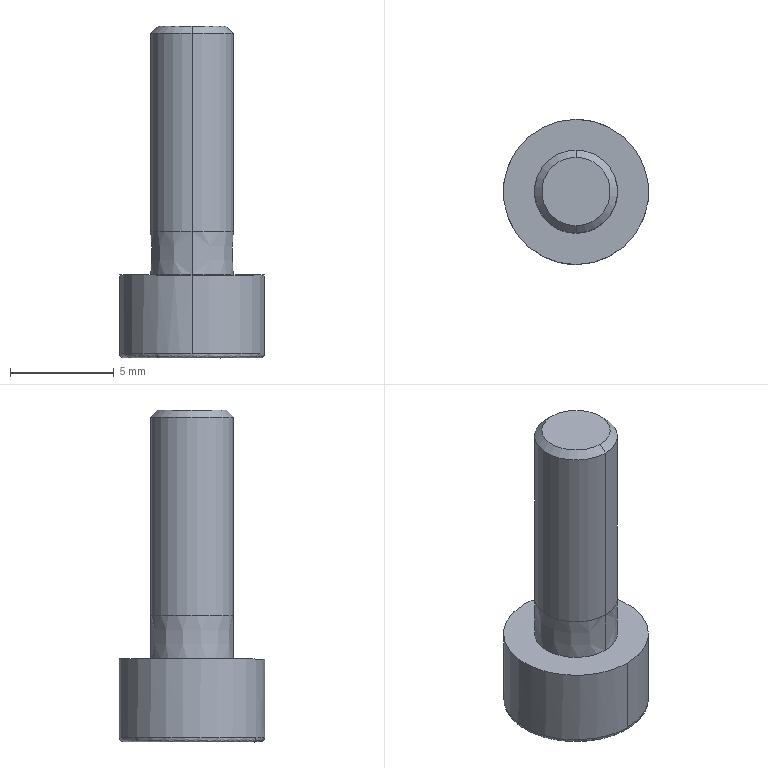Part | SolidWorks | features BaseBody 1 | 1 solid | 20 faces | box 7 x 7 x 16 mm | volume 288.226 mm3 | plane 10 | cylinder 4 | cone 4 | spline 2 | commonest cylinder face diameters 4 x2 7 x2
STEP:
#1=CARTESIAN_POINT('',(490.946,-51.279,245.744));
#2=VERTEX_POINT('',#1);
#3=CARTESIAN_POINT('',(489.266,-50.849,245.744));
#4=VERTEX_POINT('',#3);
#5=CARTESIAN_POINT('',(489.266,-54.349,245.744));
#6=DIRECTION('',(0.000000004,-0.00000001,1.));
#7=DIRECTION('',(0.,-1.,-0.00000001));
#8=AXIS2_PLACEMENT_3D('',#5,#6,#7);
#9=CIRCLE('',#8,3.5);
#10=EDGE_CURVE('',#2,#4,#9,.T.);
#11=ORIENTED_EDGE('',*,*,#10,.F.);
#12=CARTESIAN_POINT('',(490.85,-51.454,245.544));
#13=VERTEX_POINT('',#12);
#14=CARTESIAN_POINT('',(490.85,-51.454,245.744));
#15=DIRECTION('',(-0.8773,0.4799,0.000000008));
#16=DIRECTION('',(0.4799,0.8773,0.000000006));
#17=AXIS2_PLACEMENT_3D('',#14,#15,#16);
#18=CIRCLE('',#17,0.2);
#19=EDGE_CURVE('',#2,#13,#18,.T.);
#20=ORIENTED_EDGE('',*,*,#19,.T.);
#21=CARTESIAN_POINT('',(487.682,-57.244,245.544));
#22=VERTEX_POINT('',#21);
#23=CARTESIAN_POINT('',(490.85,-51.454,245.544));
#24=CARTESIAN_POINT('',(485.059,-48.287,245.544));
#25=CARTESIAN_POINT('',(481.892,-54.077,245.544));
#26=CARTESIAN_POINT('',(487.682,-57.244,245.544));
#27=(BOUNDED_CURVE()B_SPLINE_CURVE(3,(#23,#24,#25,#26),.UNSPECIFIED.,.F.,.T.)B_SPLINE_CURVE_WITH_KNOTS((4,4),(0.,1.),.UNSPECIFIED.)CURVE()GEOMETRIC_REPRESENTATION_ITEM()RATIONAL_B_SPLINE_CURVE((1.,0.3333,0.3333,1.))REPRESENTATION_ITEM(''));
#28=EDGE_CURVE('',#13,#22,#27,.T.);
#29=ORIENTED_EDGE('',*,*,#28,.T.);
#30=CARTESIAN_POINT('',(487.586,-57.42,245.744));
#31=VERTEX_POINT('',#30);
#32=CARTESIAN_POINT('',(487.682,-57.244,245.744));
#33=DIRECTION('',(0.8773,-0.4799,-0.000000008));
#34=DIRECTION('',(-0.4799,-0.8773,-0.000000006));
#35=AXIS2_PLACEMENT_3D('',#32,#33,#34);
#36=CIRCLE('',#35,0.2);
#37=EDGE_CURVE('',#31,#22,#36,.T.);
#38=ORIENTED_EDGE('',*,*,#37,.F.);
#39=CARTESIAN_POINT('',(489.266,-54.349,245.744));
#40=DIRECTION('',(0.000000004,-0.00000001,1.));
#41=DIRECTION('',(0.,-1.,-0.00000001));
#42=AXIS2_PLACEMENT_3D('',#39,#40,#41);
#43=CIRCLE('',#42,3.5);
#44=EDGE_CURVE('',#4,#31,#43,.T.);
#45=ORIENTED_EDGE('',*,*,#44,.F.);
#46=EDGE_LOOP('',(#11,#20,#29,#38,#45));
#47=FACE_OUTER_BOUND('',#46,.T.);
#48=CARTESIAN_POINT('',(490.946,-51.279,245.744));
#49=CARTESIAN_POINT('',(484.804,-47.919,245.744));
#50=CARTESIAN_POINT('',(481.445,-54.06,245.744));
#51=CARTESIAN_POINT('',(487.586,-57.42,245.744));
#52=CARTESIAN_POINT('',(490.946,-51.279,245.627));
#53=CARTESIAN_POINT('',(484.804,-47.919,245.627));
#54=CARTESIAN_POINT('',(481.445,-54.06,245.627));
#55=CARTESIAN_POINT('',(487.586,-57.42,245.627));
#56=CARTESIAN_POINT('',(490.906,-51.351,245.544));
#57=CARTESIAN_POINT('',(484.91,-48.071,245.544));
#58=CARTESIAN_POINT('',(481.63,-54.067,245.544));
#59=CARTESIAN_POINT('',(487.626,-57.347,245.544));
#60=CARTESIAN_POINT('',(490.85,-51.454,245.544));
#61=CARTESIAN_POINT('',(485.059,-48.287,245.544));
#62=CARTESIAN_POINT('',(481.892,-54.077,245.544));
#63=CARTESIAN_POINT('',(487.682,-57.244,245.544));
#64=(BOUNDED_SURFACE()B_SPLINE_SURFACE(3,3,((#48,#49,#50,#51),(#52,#53,#54,#55),(#56,#57,#58,#59),(#60,#61,#62,#63)),.UNSPECIFIED.,.F.,.F.,.F.)B_SPLINE_SURFACE_WITH_KNOTS((4,4),(4,4),(0.,1.),(0.,1.),.UNSPECIFIED.)GEOMETRIC_REPRESENTATION_ITEM()RATIONAL_B_SPLINE_SURFACE(((1.,0.3333,0.3333,1.),(0.8047,0.2682,0.2682,0.8047),(0.8047,0.2682,0.2682,0.8047),(1.,0.3333,0.3333,1.)))REPRESENTATION_ITEM('')SURFACE());
#65=ADVANCED_FACE('',(#47),#64,.T.);
#66=CARTESIAN_POINT('',(489.266,-56.349,251.644));
#67=VERTEX_POINT('',#66);
#68=CARTESIAN_POINT('',(489.266,-52.349,251.644));
#69=VERTEX_POINT('',#68);
#70=CARTESIAN_POINT('',(489.266,-54.349,251.644));
#71=DIRECTION('',(0.000000004,-0.00000001,1.));
#72=DIRECTION('',(0.,-1.,-0.00000001));
#73=AXIS2_PLACEMENT_3D('',#70,#71,#72);
#74=CIRCLE('',#73,2.);
#75=EDGE_CURVE('',#67,#69,#74,.T.);
#76=ORIENTED_EDGE('',*,*,#75,.T.);
#77=CARTESIAN_POINT('',(489.266,-52.349,261.194));
#78=VERTEX_POINT('',#77);
#79=CARTESIAN_POINT('',(489.266,-52.349,256.419));
#80=DIRECTION('',(0.000000004,-0.00000001,1.));
#81=VECTOR('',#80,1000.);
#82=LINE('',#79,#81);
#83=EDGE_CURVE('',#69,#78,#82,.T.);
#84=ORIENTED_EDGE('',*,*,#83,.T.);
#85=CARTESIAN_POINT('',(489.266,-56.349,261.194));
#86=VERTEX_POINT('',#85);
#87=CARTESIAN_POINT('',(489.266,-54.349,261.194));
#88=DIRECTION('',(-0.000000004,0.00000001,-1.));
#89=DIRECTION('',(0.,-1.,-0.00000001));
#90=AXIS2_PLACEMENT_3D('',#87,#88,#89);
#91=CIRCLE('',#90,2.);
#92=EDGE_CURVE('',#78,#86,#91,.T.);
#93=ORIENTED_EDGE('',*,*,#92,.T.);
#94=CARTESIAN_POINT('',(489.266,-56.349,256.419));
#95=DIRECTION('',(0.000000004,-0.00000001,1.));
#96=VECTOR('',#95,1000.);
#97=LINE('',#94,#96);
#98=EDGE_CURVE('',#67,#86,#97,.T.);
#99=ORIENTED_EDGE('',*,*,#98,.F.);
#100=EDGE_LOOP('',(#76,#84,#93,#99));
#101=FACE_OUTER_BOUND('',#100,.T.);
#102=CARTESIAN_POINT('',(489.266,-54.349,256.419));
#103=DIRECTION('',(0.000000004,-0.00000001,1.));
#104=DIRECTION('',(0.,-1.,-0.00000001));
#105=AXIS2_PLACEMENT_3D('',#102,#103,#104);
#106=CYLINDRICAL_SURFACE('',#105,2.);
#107=ADVANCED_FACE('',(#101),#106,.T.);
#108=CARTESIAN_POINT('',(489.266,-56.348,249.544));
#109=VERTEX_POINT('',#108);
#110=CARTESIAN_POINT('',(489.266,-52.35,249.544));
#111=VERTEX_POINT('',#110);
#112=CARTESIAN_POINT('',(489.266,-54.349,249.544));
#113=DIRECTION('',(0.000000004,-0.00000001,1.));
#114=DIRECTION('',(0.,-1.,-0.00000001));
#115=AXIS2_PLACEMENT_3D('',#112,#113,#114);
#116=CIRCLE('',#115,1.999);
#117=EDGE_CURVE('',#109,#111,#116,.T.);
#118=ORIENTED_EDGE('',*,*,#117,.T.);
#119=CARTESIAN_POINT('',(489.266,-52.349,251.644));
#120=DIRECTION('',(0.000000004,0.0004762,1.));
#121=VECTOR('',#120,1000.);
#122=LINE('',#119,#121);
#123=EDGE_CURVE('',#111,#69,#122,.T.);
#124=ORIENTED_EDGE('',*,*,#123,.T.);
#125=ORIENTED_EDGE('',*,*,#75,.F.);
#126=CARTESIAN_POINT('',(489.266,-56.349,251.644));
#127=DIRECTION('',(0.000000004,-0.0004762,1.));
#128=VECTOR('',#127,1000.);
#129=LINE('',#126,#128);
#130=EDGE_CURVE('',#109,#67,#129,.T.);
#131=ORIENTED_EDGE('',*,*,#130,.F.);
#132=EDGE_LOOP('',(#118,#124,#125,#131));
#133=FACE_OUTER_BOUND('',#132,.T.);
#134=CARTESIAN_POINT('',(489.266,-54.349,251.644));
#135=DIRECTION('',(0.000000004,-0.00000001,1.));
#136=DIRECTION('',(0.,-1.,-0.00000001));
#137=AXIS2_PLACEMENT_3D('',#134,#135,#136);
#138=CONICAL_SURFACE('',#137,2.,0.0004762);
#139=ADVANCED_FACE('',(#133),#138,.T.);
#140=CARTESIAN_POINT('',(489.266,-52.699,261.544));
#141=VERTEX_POINT('',#140);
#142=CARTESIAN_POINT('',(489.266,-55.999,261.544));
#143=VERTEX_POINT('',#142);
#144=CARTESIAN_POINT('',(489.266,-54.349,261.544));
#145=DIRECTION('',(-0.000000004,0.00000001,-1.));
#146=DIRECTION('',(0.,1.,0.00000001));
#147=AXIS2_PLACEMENT_3D('',#144,#145,#146);
#148=CIRCLE('',#147,1.65);
#149=EDGE_CURVE('',#141,#143,#148,.T.);
#150=ORIENTED_EDGE('',*,*,#149,.T.);
#151=CARTESIAN_POINT('',(489.266,-56.349,261.194));
#152=DIRECTION('',(-0.000000003,-0.7071,-0.7071));
#153=VECTOR('',#152,1000.);
#154=LINE('',#151,#153);
#155=EDGE_CURVE('',#143,#86,#154,.T.);
#156=ORIENTED_EDGE('',*,*,#155,.T.);
#157=ORIENTED_EDGE('',*,*,#92,.F.);
#158=CARTESIAN_POINT('',(489.266,-52.349,261.194));
#159=DIRECTION('',(-0.000000003,0.7071,-0.7071));
#160=VECTOR('',#159,1000.);
#161=LINE('',#158,#160);
#162=EDGE_CURVE('',#141,#78,#161,.T.);
#163=ORIENTED_EDGE('',*,*,#162,.F.);
#164=EDGE_LOOP('',(#150,#156,#157,#163));
#165=FACE_OUTER_BOUND('',#164,.T.);
#166=CARTESIAN_POINT('',(489.266,-54.349,261.194));
#167=DIRECTION('',(-0.000000004,0.00000001,-1.));
#168=DIRECTION('',(0.,1.,0.00000001));
#169=AXIS2_PLACEMENT_3D('',#166,#167,#168);
#170=CONICAL_SURFACE('',#169,2.,0.7854);
#171=ADVANCED_FACE('',(#165),#170,.T.);
#172=CARTESIAN_POINT('',(489.266,-57.849,245.744));
#173=VERTEX_POINT('',#172);
#174=CARTESIAN_POINT('',(489.266,-54.349,245.744));
#175=DIRECTION('',(0.000000004,-0.00000001,1.));
#176=DIRECTION('',(0.,-1.,-0.00000001));
#177=AXIS2_PLACEMENT_3D('',#174,#175,#176);
#178=CIRCLE('',#177,3.5);
#179=EDGE_CURVE('',#173,#2,#178,.T.);
#180=ORIENTED_EDGE('',*,*,#179,.T.);
#181=ORIENTED_EDGE('',*,*,#10,.T.);
#182=CARTESIAN_POINT('',(489.266,-50.849,249.544));
#183=VERTEX_POINT('',#182);
#184=CARTESIAN_POINT('',(489.266,-50.849,247.644));
#185=DIRECTION('',(0.000000004,-0.00000001,1.));
#186=VECTOR('',#185,1000.);
#187=LINE('',#184,#186);
#188=EDGE_CURVE('',#4,#183,#187,.T.);
#189=ORIENTED_EDGE('',*,*,#188,.T.);
#190=CARTESIAN_POINT('',(489.266,-57.849,249.544));
#191=VERTEX_POINT('',#190);
#192=CARTESIAN_POINT('',(489.266,-54.349,249.544));
#193=DIRECTION('',(0.000000004,-0.00000001,1.));
#194=DIRECTION('',(0.,-1.,-0.00000001));
#195=AXIS2_PLACEMENT_3D('',#192,#193,#194);
#196=CIRCLE('',#195,3.5);
#197=EDGE_CURVE('',#191,#183,#196,.T.);
#198=ORIENTED_EDGE('',*,*,#197,.F.);
#199=CARTESIAN_POINT('',(489.266,-57.849,247.644));
#200=DIRECTION('',(0.000000004,-0.00000001,1.));
#201=VECTOR('',#200,1000.);
#202=LINE('',#199,#201);
#203=EDGE_CURVE('',#173,#191,#202,.T.);
#204=ORIENTED_EDGE('',*,*,#203,.F.);
#205=EDGE_LOOP('',(#180,#181,#189,#198,#204));
#206=FACE_OUTER_BOUND('',#205,.T.);
#207=CARTESIAN_POINT('',(489.266,-54.349,247.644));
#208=DIRECTION('',(0.000000004,-0.00000001,1.));
#209=DIRECTION('',(0.,-1.,-0.00000001));
#210=AXIS2_PLACEMENT_3D('',#207,#208,#209);
#211=CYLINDRICAL_SURFACE('',#210,3.5);
#212=ADVANCED_FACE('',(#206),#211,.T.);
#213=ORIENTED_EDGE('',*,*,#83,.F.);
#214=CARTESIAN_POINT('',(489.266,-54.349,251.644));
#215=DIRECTION('',(0.000000004,-0.00000001,1.));
#216=DIRECTION('',(0.,-1.,-0.00000001));
#217=AXIS2_PLACEMENT_3D('',#214,#215,#216);
#218=CIRCLE('',#217,2.);
#219=EDGE_CURVE('',#69,#67,#218,.T.);
#220=ORIENTED_EDGE('',*,*,#219,.T.);
#221=ORIENTED_EDGE('',*,*,#98,.T.);
#222=CARTESIAN_POINT('',(489.266,-54.349,261.194));
#223=DIRECTION('',(-0.000000004,0.00000001,-1.));
#224=DIRECTION('',(0.,-1.,-0.00000001));
#225=AXIS2_PLACEMENT_3D('',#222,#223,#224);
#226=CIRCLE('',#225,2.);
#227=EDGE_CURVE('',#86,#78,#226,.T.);
#228=ORIENTED_EDGE('',*,*,#227,.T.);
#229=EDGE_LOOP('',(#213,#220,#221,#228));
#230=FACE_OUTER_BOUND('',#229,.T.);
#231=CARTESIAN_POINT('',(489.266,-54.349,256.419));
#232=DIRECTION('',(0.000000004,-0.00000001,1.));
#233=DIRECTION('',(0.,-1.,-0.00000001));
#234=AXIS2_PLACEMENT_3D('',#231,#232,#233);
#235=CYLINDRICAL_SURFACE('',#234,2.);
#236=ADVANCED_FACE('',(#230),#235,.T.);
#237=ORIENTED_EDGE('',*,*,#123,.F.);
#238=CARTESIAN_POINT('',(489.266,-54.349,249.544));
#239=DIRECTION('',(0.000000004,-0.00000001,1.));
#240=DIRECTION('',(0.,-1.,-0.00000001));
#241=AXIS2_PLACEMENT_3D('',#238,#239,#240);
#242=CIRCLE('',#241,1.999);
#243=EDGE_CURVE('',#111,#109,#242,.T.);
#244=ORIENTED_EDGE('',*,*,#243,.T.);
#245=ORIENTED_EDGE('',*,*,#130,.T.);
#246=ORIENTED_EDGE('',*,*,#219,.F.);
#247=EDGE_LOOP('',(#237,#244,#245,#246));
#248=FACE_OUTER_BOUND('',#247,.T.);
#249=CARTESIAN_POINT('',(489.266,-54.349,251.644));
#250=DIRECTION('',(0.000000004,-0.00000001,1.));
#251=DIRECTION('',(0.,-1.,-0.00000001));
#252=AXIS2_PLACEMENT_3D('',#249,#250,#251);
#253=CONICAL_SURFACE('',#252,2.,0.0004762);
#254=ADVANCED_FACE('',(#248),#253,.T.);
#255=ORIENTED_EDGE('',*,*,#155,.F.);
#256=CARTESIAN_POINT('',(489.266,-54.349,261.544));
#257=DIRECTION('',(-0.000000004,0.00000001,-1.));
#258=DIRECTION('',(0.,1.,0.00000001));
#259=AXIS2_PLACEMENT_3D('',#256,#257,#258);
#260=CIRCLE('',#259,1.65);
#261=EDGE_CURVE('',#143,#141,#260,.T.);
#262=ORIENTED_EDGE('',*,*,#261,.T.);
#263=ORIENTED_EDGE('',*,*,#162,.T.);
#264=ORIENTED_EDGE('',*,*,#227,.F.);
#265=EDGE_LOOP('',(#255,#262,#263,#264));
#266=FACE_OUTER_BOUND('',#265,.T.);
#267=CARTESIAN_POINT('',(489.266,-54.349,261.194));
#268=DIRECTION('',(-0.000000004,0.00000001,-1.));
#269=DIRECTION('',(0.,1.,0.00000001));
#270=AXIS2_PLACEMENT_3D('',#267,#268,#269);
#271=CONICAL_SURFACE('',#270,2.,0.7854);
#272=ADVANCED_FACE('',(#266),#271,.T.);
#273=ORIENTED_EDGE('',*,*,#117,.F.);
#274=ORIENTED_EDGE('',*,*,#243,.F.);
#275=EDGE_LOOP('',(#273,#274));
#276=FACE_BOUND('',#275,.T.);
#277=ORIENTED_EDGE('',*,*,#197,.T.);
#278=CARTESIAN_POINT('',(489.266,-54.349,249.544));
#279=DIRECTION('',(0.000000004,-0.00000001,1.));
#280=DIRECTION('',(0.,-1.,-0.00000001));
#281=AXIS2_PLACEMENT_3D('',#278,#279,#280);
#282=CIRCLE('',#281,3.5);
#283=EDGE_CURVE('',#183,#191,#282,.T.);
#284=ORIENTED_EDGE('',*,*,#283,.T.);
#285=EDGE_LOOP('',(#277,#284));
#286=FACE_OUTER_BOUND('',#285,.T.);
#287=CARTESIAN_POINT('',(488.426,-55.884,249.544));
#288=DIRECTION('',(0.000000004,-0.00000001,1.));
#289=DIRECTION('',(0.,-1.,-0.00000001));
#290=AXIS2_PLACEMENT_3D('',#287,#288,#289);
#291=PLANE('',#290);
#292=ADVANCED_FACE('',(#276,#286),#291,.T.);
#293=ORIENTED_EDGE('',*,*,#149,.F.);
#294=ORIENTED_EDGE('',*,*,#261,.F.);
#295=EDGE_LOOP('',(#293,#294));
#296=FACE_OUTER_BOUND('',#295,.T.);
#297=CARTESIAN_POINT('',(488.87,-55.073,261.544));
#298=DIRECTION('',(0.000000004,-0.00000001,1.));
#299=DIRECTION('',(0.,-1.,-0.00000001));
#300=AXIS2_PLACEMENT_3D('',#297,#298,#299);
#301=PLANE('',#300);
#302=ADVANCED_FACE('',(#296),#301,.T.);
#303=ORIENTED_EDGE('',*,*,#188,.F.);
#304=ORIENTED_EDGE('',*,*,#44,.T.);
#305=CARTESIAN_POINT('',(489.266,-54.349,245.744));
#306=DIRECTION('',(0.000000004,-0.00000001,1.));
#307=DIRECTION('',(0.,-1.,-0.00000001));
#308=AXIS2_PLACEMENT_3D('',#305,#306,#307);
#309=CIRCLE('',#308,3.5);
#310=EDGE_CURVE('',#31,#173,#309,.T.);
#311=ORIENTED_EDGE('',*,*,#310,.T.);
#312=ORIENTED_EDGE('',*,*,#203,.T.);
#313=ORIENTED_EDGE('',*,*,#283,.F.);
#314=EDGE_LOOP('',(#303,#304,#311,#312,#313));
#315=FACE_OUTER_BOUND('',#314,.T.);
#316=CARTESIAN_POINT('',(489.266,-54.349,247.644));
#317=DIRECTION('',(0.000000004,-0.00000001,1.));
#318=DIRECTION('',(0.,-1.,-0.00000001));
#319=AXIS2_PLACEMENT_3D('',#316,#317,#318);
#320=CYLINDRICAL_SURFACE('',#319,3.5);
#321=ADVANCED_FACE('',(#315),#320,.T.);
#322=ORIENTED_EDGE('',*,*,#19,.F.);
#323=ORIENTED_EDGE('',*,*,#179,.F.);
#324=ORIENTED_EDGE('',*,*,#310,.F.);
#325=ORIENTED_EDGE('',*,*,#37,.T.);
#326=CARTESIAN_POINT('',(487.682,-57.244,245.544));
#327=CARTESIAN_POINT('',(493.472,-60.412,245.544));
#328=CARTESIAN_POINT('',(496.64,-54.621,245.544));
#329=CARTESIAN_POINT('',(490.85,-51.454,245.544));
#330=(BOUNDED_CURVE()B_SPLINE_CURVE(3,(#326,#327,#328,#329),.UNSPECIFIED.,.F.,.T.)B_SPLINE_CURVE_WITH_KNOTS((4,4),(0.,1.),.UNSPECIFIED.)CURVE()GEOMETRIC_REPRESENTATION_ITEM()RATIONAL_B_SPLINE_CURVE((1.,0.3333,0.3333,1.))REPRESENTATION_ITEM(''));
#331=EDGE_CURVE('',#22,#13,#330,.T.);
#332=ORIENTED_EDGE('',*,*,#331,.T.);
#333=EDGE_LOOP('',(#322,#323,#324,#325,#332));
#334=FACE_OUTER_BOUND('',#333,.T.);
#335=CARTESIAN_POINT('',(487.586,-57.42,245.744));
#336=CARTESIAN_POINT('',(493.727,-60.779,245.744));
#337=CARTESIAN_POINT('',(497.087,-54.638,245.744));
#338=CARTESIAN_POINT('',(490.946,-51.279,245.744));
#339=CARTESIAN_POINT('',(487.586,-57.42,245.627));
#340=CARTESIAN_POINT('',(493.727,-60.779,245.627));
#341=CARTESIAN_POINT('',(497.087,-54.638,245.627));
#342=CARTESIAN_POINT('',(490.946,-51.279,245.627));
#343=CARTESIAN_POINT('',(487.626,-57.347,245.544));
#344=CARTESIAN_POINT('',(493.622,-60.627,245.544));
#345=CARTESIAN_POINT('',(496.902,-54.631,245.544));
#346=CARTESIAN_POINT('',(490.906,-51.351,245.544));
#347=CARTESIAN_POINT('',(487.682,-57.244,245.544));
#348=CARTESIAN_POINT('',(493.472,-60.412,245.544));
#349=CARTESIAN_POINT('',(496.64,-54.621,245.544));
#350=CARTESIAN_POINT('',(490.85,-51.454,245.544));
#351=(BOUNDED_SURFACE()B_SPLINE_SURFACE(3,3,((#335,#336,#337,#338),(#339,#340,#341,#342),(#343,#344,#345,#346),(#347,#348,#349,#350)),.UNSPECIFIED.,.F.,.F.,.F.)B_SPLINE_SURFACE_WITH_KNOTS((4,4),(4,4),(0.,1.),(0.,1.),.UNSPECIFIED.)GEOMETRIC_REPRESENTATION_ITEM()RATIONAL_B_SPLINE_SURFACE(((1.,0.3333,0.3333,1.),(0.8047,0.2682,0.2682,0.8047),(0.8047,0.2682,0.2682,0.8047),(1.,0.3333,0.3333,1.)))REPRESENTATION_ITEM('')SURFACE());
#352=ADVANCED_FACE('',(#334),#351,.T.);
#353=ORIENTED_EDGE('',*,*,#28,.F.);
#354=ORIENTED_EDGE('',*,*,#331,.F.);
#355=EDGE_LOOP('',(#353,#354));
#356=FACE_OUTER_BOUND('',#355,.T.);
#357=CARTESIAN_POINT('',(490.997,-54.309,245.544));
#358=VERTEX_POINT('',#357);
#359=CARTESIAN_POINT('',(490.097,-52.83,245.544));
#360=VERTEX_POINT('',#359);
#361=CARTESIAN_POINT('',(490.097,-52.83,245.544));
#362=DIRECTION('',(-0.5198,0.8543,0.));
#363=VECTOR('',#362,1000.);
#364=LINE('',#361,#363);
#365=EDGE_CURVE('',#358,#360,#364,.T.);
#366=ORIENTED_EDGE('',*,*,#365,.T.);
#367=CARTESIAN_POINT('',(488.366,-52.87,245.544));
#368=VERTEX_POINT('',#367);
#369=CARTESIAN_POINT('',(490.097,-52.83,245.544));
#370=DIRECTION('',(-0.9997,-0.02304,0.000000004));
#371=VECTOR('',#370,1000.);
#372=LINE('',#369,#371);
#373=EDGE_CURVE('',#360,#368,#372,.T.);
#374=ORIENTED_EDGE('',*,*,#373,.T.);
#375=CARTESIAN_POINT('',(487.534,-54.389,245.544));
#376=VERTEX_POINT('',#375);
#377=CARTESIAN_POINT('',(487.534,-54.389,245.544));
#378=DIRECTION('',(-0.4799,-0.8773,0.));
#379=VECTOR('',#378,1000.);
#380=LINE('',#377,#379);
#381=EDGE_CURVE('',#368,#376,#380,.T.);
#382=ORIENTED_EDGE('',*,*,#381,.T.);
#383=CARTESIAN_POINT('',(488.435,-55.869,245.544));
#384=VERTEX_POINT('',#383);
#385=CARTESIAN_POINT('',(488.435,-55.869,245.544));
#386=DIRECTION('',(0.5198,-0.8543,0.));
#387=VECTOR('',#386,1000.);
#388=LINE('',#385,#387);
#389=EDGE_CURVE('',#376,#384,#388,.T.);
#390=ORIENTED_EDGE('',*,*,#389,.T.);
#391=CARTESIAN_POINT('',(490.166,-55.829,245.544));
#392=VERTEX_POINT('',#391);
#393=CARTESIAN_POINT('',(490.166,-55.829,245.544));
#394=DIRECTION('',(0.9997,0.02304,0.));
#395=VECTOR('',#394,1000.);
#396=LINE('',#393,#395);
#397=EDGE_CURVE('',#384,#392,#396,.T.);
#398=ORIENTED_EDGE('',*,*,#397,.T.);
#399=CARTESIAN_POINT('',(490.997,-54.309,245.544));
#400=DIRECTION('',(0.4799,0.8773,0.));
#401=VECTOR('',#400,1000.);
#402=LINE('',#399,#401);
#403=EDGE_CURVE('',#392,#358,#402,.T.);
#404=ORIENTED_EDGE('',*,*,#403,.T.);
#405=EDGE_LOOP('',(#366,#374,#382,#390,#398,#404));
#406=FACE_BOUND('',#405,.T.);
#407=CARTESIAN_POINT('',(488.474,-55.797,245.544));
#408=DIRECTION('',(-0.000000004,0.00000001,-1.));
#409=DIRECTION('',(0.,1.,0.00000001));
#410=AXIS2_PLACEMENT_3D('',#407,#408,#409);
#411=PLANE('',#410);
#412=ADVANCED_FACE('',(#356,#406),#411,.T.);
#413=CARTESIAN_POINT('',(488.366,-52.87,247.544));
#414=VERTEX_POINT('',#413);
#415=CARTESIAN_POINT('',(488.366,-52.87,245.544));
#416=DIRECTION('',(0.,-0.00000001,1.));
#417=VECTOR('',#416,1000.);
#418=LINE('',#415,#417);
#419=EDGE_CURVE('',#368,#414,#418,.T.);
#420=ORIENTED_EDGE('',*,*,#419,.F.);
#421=ORIENTED_EDGE('',*,*,#373,.F.);
#422=CARTESIAN_POINT('',(490.097,-52.83,247.544));
#423=VERTEX_POINT('',#422);
#424=CARTESIAN_POINT('',(490.097,-52.83,245.544));
#425=DIRECTION('',(0.,0.00000001,-1.));
#426=VECTOR('',#425,1000.);
#427=LINE('',#424,#426);
#428=EDGE_CURVE('',#423,#360,#427,.T.);
#429=ORIENTED_EDGE('',*,*,#428,.F.);
#430=CARTESIAN_POINT('',(488.366,-52.87,247.544));
#431=DIRECTION('',(0.9997,0.02304,0.));
#432=VECTOR('',#431,1000.);
#433=LINE('',#430,#432);
#434=EDGE_CURVE('',#414,#423,#433,.T.);
#435=ORIENTED_EDGE('',*,*,#434,.F.);
#436=EDGE_LOOP('',(#420,#421,#429,#435));
#437=FACE_OUTER_BOUND('',#436,.T.);
#438=CARTESIAN_POINT('',(488.366,-52.87,245.544));
#439=DIRECTION('',(-0.02304,0.9997,0.00000001));
#440=DIRECTION('',(-0.9997,-0.02304,0.));
#441=AXIS2_PLACEMENT_3D('',#438,#439,#440);
#442=PLANE('',#441);
#443=ADVANCED_FACE('',(#437),#442,.F.);
#444=CARTESIAN_POINT('',(490.166,-55.829,247.544));
#445=VERTEX_POINT('',#444);
#446=CARTESIAN_POINT('',(488.435,-55.869,247.544));
#447=VERTEX_POINT('',#446);
#448=CARTESIAN_POINT('',(490.166,-55.829,247.544));
#449=DIRECTION('',(-0.9997,-0.02304,0.));
#450=VECTOR('',#449,1000.);
#451=LINE('',#448,#450);
#452=EDGE_CURVE('',#445,#447,#451,.T.);
#453=ORIENTED_EDGE('',*,*,#452,.T.);
#454=CARTESIAN_POINT('',(487.534,-54.389,247.544));
#455=VERTEX_POINT('',#454);
#456=CARTESIAN_POINT('',(488.435,-55.869,247.544));
#457=DIRECTION('',(-0.5198,0.8543,0.));
#458=VECTOR('',#457,1000.);
#459=LINE('',#456,#458);
#460=EDGE_CURVE('',#447,#455,#459,.T.);
#461=ORIENTED_EDGE('',*,*,#460,.T.);
#462=CARTESIAN_POINT('',(487.534,-54.389,247.544));
#463=DIRECTION('',(0.4799,0.8773,0.000000006));
#464=VECTOR('',#463,1000.);
#465=LINE('',#462,#464);
#466=EDGE_CURVE('',#455,#414,#465,.T.);
#467=ORIENTED_EDGE('',*,*,#466,.T.);
#468=ORIENTED_EDGE('',*,*,#434,.T.);
#469=CARTESIAN_POINT('',(490.997,-54.309,247.544));
#470=VERTEX_POINT('',#469);
#471=CARTESIAN_POINT('',(490.097,-52.83,247.544));
#472=DIRECTION('',(0.5198,-0.8543,-0.000000011));
#473=VECTOR('',#472,1000.);
#474=LINE('',#471,#473);
#475=EDGE_CURVE('',#423,#470,#474,.T.);
#476=ORIENTED_EDGE('',*,*,#475,.T.);
#477=CARTESIAN_POINT('',(490.997,-54.309,247.544));
#478=DIRECTION('',(-0.4799,-0.8773,0.));
#479=VECTOR('',#478,1000.);
#480=LINE('',#477,#479);
#481=EDGE_CURVE('',#470,#445,#480,.T.);
#482=ORIENTED_EDGE('',*,*,#481,.T.);
#483=EDGE_LOOP('',(#453,#461,#467,#468,#476,#482));
#484=FACE_OUTER_BOUND('',#483,.T.);
#485=CARTESIAN_POINT('',(489.266,-54.349,247.544));
#486=DIRECTION('',(-0.000000004,0.00000001,-1.));
#487=DIRECTION('',(0.,1.,0.00000001));
#488=AXIS2_PLACEMENT_3D('',#485,#486,#487);
#489=PLANE('',#488);
#490=ADVANCED_FACE('',(#484),#489,.T.);
#491=CARTESIAN_POINT('',(487.534,-54.389,245.544));
#492=DIRECTION('',(0.000000007,-0.000000004,1.));
#493=VECTOR('',#492,1000.);
#494=LINE('',#491,#493);
#495=EDGE_CURVE('',#376,#455,#494,.T.);
#496=ORIENTED_EDGE('',*,*,#495,.F.);
#497=ORIENTED_EDGE('',*,*,#381,.F.);
#498=ORIENTED_EDGE('',*,*,#419,.T.);
#499=ORIENTED_EDGE('',*,*,#466,.F.);
#500=EDGE_LOOP('',(#496,#497,#498,#499));
#501=FACE_OUTER_BOUND('',#500,.T.);
#502=CARTESIAN_POINT('',(487.534,-54.389,245.544));
#503=DIRECTION('',(-0.8773,0.4799,0.000000008));
#504=DIRECTION('',(-0.4799,-0.8773,0.));
#505=AXIS2_PLACEMENT_3D('',#502,#503,#504);
#506=PLANE('',#505);
#507=ADVANCED_FACE('',(#501),#506,.F.);
#508=ORIENTED_EDGE('',*,*,#428,.T.);
#509=ORIENTED_EDGE('',*,*,#365,.F.);
#510=CARTESIAN_POINT('',(490.997,-54.309,245.544));
#511=DIRECTION('',(0.000000001,0.000000001,-1.));
#512=VECTOR('',#511,1000.);
#513=LINE('',#510,#512);
#514=EDGE_CURVE('',#470,#358,#513,.T.);
#515=ORIENTED_EDGE('',*,*,#514,.F.);
#516=ORIENTED_EDGE('',*,*,#475,.F.);
#517=EDGE_LOOP('',(#508,#509,#515,#516));
#518=FACE_OUTER_BOUND('',#517,.T.);
#519=CARTESIAN_POINT('',(490.097,-52.83,245.544));
#520=DIRECTION('',(0.8543,0.5198,0.000000001));
#521=DIRECTION('',(-0.5198,0.8543,0.));
#522=AXIS2_PLACEMENT_3D('',#519,#520,#521);
#523=PLANE('',#522);
#524=ADVANCED_FACE('',(#518),#523,.F.);
#525=CARTESIAN_POINT('',(488.435,-55.869,245.544));
#526=DIRECTION('',(-0.000000001,-0.000000001,1.));
#527=VECTOR('',#526,1000.);
#528=LINE('',#525,#527);
#529=EDGE_CURVE('',#384,#447,#528,.T.);
#530=ORIENTED_EDGE('',*,*,#529,.F.);
#531=ORIENTED_EDGE('',*,*,#389,.F.);
#532=ORIENTED_EDGE('',*,*,#495,.T.);
#533=ORIENTED_EDGE('',*,*,#460,.F.);
#534=EDGE_LOOP('',(#530,#531,#532,#533));
#535=FACE_OUTER_BOUND('',#534,.T.);
#536=CARTESIAN_POINT('',(488.435,-55.869,245.544));
#537=DIRECTION('',(-0.8543,-0.5198,-0.000000001));
#538=DIRECTION('',(0.5198,-0.8543,0.));
#539=AXIS2_PLACEMENT_3D('',#536,#537,#538);
#540=PLANE('',#539);
#541=ADVANCED_FACE('',(#535),#540,.F.);
#542=ORIENTED_EDGE('',*,*,#514,.T.);
#543=ORIENTED_EDGE('',*,*,#403,.F.);
#544=CARTESIAN_POINT('',(490.166,-55.829,245.544));
#545=DIRECTION('',(-0.000000007,0.000000004,-1.));
#546=VECTOR('',#545,1000.);
#547=LINE('',#544,#546);
#548=EDGE_CURVE('',#445,#392,#547,.T.);
#549=ORIENTED_EDGE('',*,*,#548,.F.);
#550=ORIENTED_EDGE('',*,*,#481,.F.);
#551=EDGE_LOOP('',(#542,#543,#549,#550));
#552=FACE_OUTER_BOUND('',#551,.T.);
#553=CARTESIAN_POINT('',(490.997,-54.309,245.544));
#554=DIRECTION('',(0.8773,-0.4799,-0.000000008));
#555=DIRECTION('',(0.4799,0.8773,0.));
#556=AXIS2_PLACEMENT_3D('',#553,#554,#555);
#557=PLANE('',#556);
#558=ADVANCED_FACE('',(#552),#557,.F.);
#559=ORIENTED_EDGE('',*,*,#548,.T.);
#560=ORIENTED_EDGE('',*,*,#397,.F.);
#561=ORIENTED_EDGE('',*,*,#529,.T.);
#562=ORIENTED_EDGE('',*,*,#452,.F.);
#563=EDGE_LOOP('',(#559,#560,#561,#562));
#564=FACE_OUTER_BOUND('',#563,.T.);
#565=CARTESIAN_POINT('',(490.166,-55.829,245.544));
#566=DIRECTION('',(0.02304,-0.9997,-0.00000001));
#567=DIRECTION('',(0.9997,0.02304,0.));
#568=AXIS2_PLACEMENT_3D('',#565,#566,#567);
#569=PLANE('',#568);
#570=ADVANCED_FACE('',(#564),#569,.F.);
#571=CLOSED_SHELL('',(#65,#107,#139,#171,#212,#236,#254,#272,#292,#302,#321,#352,#412,#443,#490,#507,#524,#541,#558,#570));
#572=MANIFOLD_SOLID_BREP('',#571);
#573=CARTESIAN_POINT('',(0.,0.,0.));
#574=DIRECTION('',(0.,0.,1.));
#575=DIRECTION('',(1.,0.,0.));
#576=AXIS2_PLACEMENT_3D('',#573,#574,#575);
#577=(LENGTH_UNIT()NAMED_UNIT(*)SI_UNIT(.MILLI.,.METRE.));
#578=UNCERTAINTY_MEASURE_WITH_UNIT(LENGTH_MEASURE(0.00001),#577,'','');
#579=(NAMED_UNIT(*)PLANE_ANGLE_UNIT()SI_UNIT($,.RADIAN.));
#580=(NAMED_UNIT(*)SI_UNIT($,.STERADIAN.)SOLID_ANGLE_UNIT());
#581=(GEOMETRIC_REPRESENTATION_CONTEXT(3)GLOBAL_UNCERTAINTY_ASSIGNED_CONTEXT((#578))GLOBAL_UNIT_ASSIGNED_CONTEXT((#577,#579,#580))REPRESENTATION_CONTEXT('',''));
#582=ADVANCED_BREP_SHAPE_REPRESENTATION('',(#572,#576),#581);